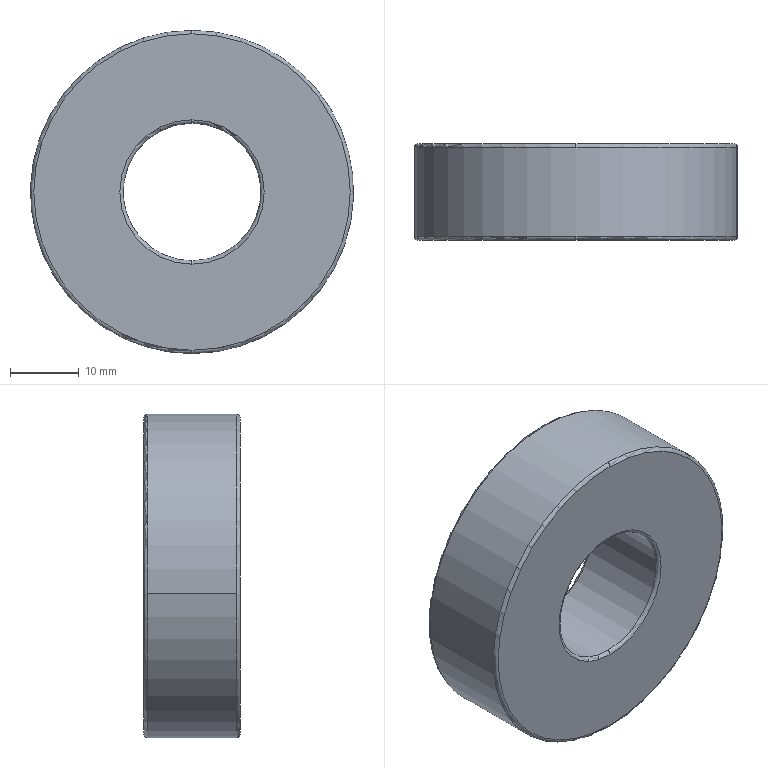Part | SolidWorks | features BaseBody 1 | 1 solid | 14 faces | box 47 x 14 x 47 mm | volume 19868 mm3 | torus 8 | cylinder 4 | plane 2 | commonest cylinder face diameters 20 x2 47 x2
STEP:
#1=CARTESIAN_POINT('',(-530.322,-112.,7.791));
#2=VERTEX_POINT('',#1);
#3=CARTESIAN_POINT('',(-530.322,-112.,28.791));
#4=VERTEX_POINT('',#3);
#5=CARTESIAN_POINT('',(-530.322,-112.,18.291));
#6=DIRECTION('',(0.,1.,0.));
#7=DIRECTION('',(0.,0.,-1.));
#8=AXIS2_PLACEMENT_3D('',#5,#6,#7);
#9=CIRCLE('',#8,10.5);
#10=EDGE_CURVE('',#2,#4,#9,.T.);
#11=ORIENTED_EDGE('',*,*,#10,.F.);
#12=CARTESIAN_POINT('',(-530.322,-111.5,8.291));
#13=VERTEX_POINT('',#12);
#14=CARTESIAN_POINT('',(-530.322,-111.5,7.791));
#15=DIRECTION('',(-1.,0.,0.));
#16=DIRECTION('',(0.,0.,1.));
#17=AXIS2_PLACEMENT_3D('',#14,#15,#16);
#18=CIRCLE('',#17,0.5);
#19=EDGE_CURVE('',#2,#13,#18,.T.);
#20=ORIENTED_EDGE('',*,*,#19,.T.);
#21=CARTESIAN_POINT('',(-540.261,-111.5,17.194));
#22=VERTEX_POINT('',#21);
#23=CARTESIAN_POINT('',(-530.322,-111.5,18.291));
#24=DIRECTION('',(0.,1.,0.));
#25=DIRECTION('',(0.,0.,-1.));
#26=AXIS2_PLACEMENT_3D('',#23,#24,#25);
#27=CIRCLE('',#26,10.);
#28=EDGE_CURVE('',#13,#22,#27,.T.);
#29=ORIENTED_EDGE('',*,*,#28,.T.);
#30=CARTESIAN_POINT('',(-530.322,-111.5,28.291));
#31=VERTEX_POINT('',#30);
#32=CARTESIAN_POINT('',(-530.322,-111.5,18.291));
#33=DIRECTION('',(0.,1.,0.));
#34=DIRECTION('',(0.,0.,-1.));
#35=AXIS2_PLACEMENT_3D('',#32,#33,#34);
#36=CIRCLE('',#35,10.);
#37=EDGE_CURVE('',#22,#31,#36,.T.);
#38=ORIENTED_EDGE('',*,*,#37,.T.);
#39=CARTESIAN_POINT('',(-530.322,-111.5,28.791));
#40=DIRECTION('',(1.,0.,0.));
#41=DIRECTION('',(0.,0.,-1.));
#42=AXIS2_PLACEMENT_3D('',#39,#40,#41);
#43=CIRCLE('',#42,0.5);
#44=EDGE_CURVE('',#4,#31,#43,.T.);
#45=ORIENTED_EDGE('',*,*,#44,.F.);
#46=EDGE_LOOP('',(#11,#20,#29,#38,#45));
#47=FACE_OUTER_BOUND('',#46,.T.);
#48=CARTESIAN_POINT('',(-530.322,-111.5,18.291));
#49=DIRECTION('',(0.,-1.,0.));
#50=DIRECTION('',(0.,0.,1.));
#51=AXIS2_PLACEMENT_3D('',#48,#49,#50);
#52=TOROIDAL_SURFACE('',#51,10.5,0.5);
#53=ADVANCED_FACE('',(#47),#52,.T.);
#54=CARTESIAN_POINT('',(-553.68,-111.5,15.712));
#55=VERTEX_POINT('',#54);
#56=CARTESIAN_POINT('',(-530.322,-111.5,-5.209));
#57=VERTEX_POINT('',#56);
#58=CARTESIAN_POINT('',(-530.322,-111.5,18.291));
#59=DIRECTION('',(0.,-1.,0.));
#60=DIRECTION('',(0.,0.,-1.));
#61=AXIS2_PLACEMENT_3D('',#58,#59,#60);
#62=CIRCLE('',#61,23.5);
#63=EDGE_CURVE('',#55,#57,#62,.T.);
#64=ORIENTED_EDGE('',*,*,#63,.T.);
#65=CARTESIAN_POINT('',(-530.322,-112.,-4.709));
#66=VERTEX_POINT('',#65);
#67=CARTESIAN_POINT('',(-530.322,-111.5,-4.709));
#68=DIRECTION('',(-1.,0.,0.));
#69=DIRECTION('',(0.,0.,1.));
#70=AXIS2_PLACEMENT_3D('',#67,#68,#69);
#71=CIRCLE('',#70,0.5);
#72=EDGE_CURVE('',#57,#66,#71,.T.);
#73=ORIENTED_EDGE('',*,*,#72,.T.);
#74=CARTESIAN_POINT('',(-530.322,-112.,41.291));
#75=VERTEX_POINT('',#74);
#76=CARTESIAN_POINT('',(-530.322,-112.,18.291));
#77=DIRECTION('',(0.,-1.,0.));
#78=DIRECTION('',(0.,0.,-1.));
#79=AXIS2_PLACEMENT_3D('',#76,#77,#78);
#80=CIRCLE('',#79,23.);
#81=EDGE_CURVE('',#75,#66,#80,.T.);
#82=ORIENTED_EDGE('',*,*,#81,.F.);
#83=CARTESIAN_POINT('',(-530.322,-111.5,41.791));
#84=VERTEX_POINT('',#83);
#85=CARTESIAN_POINT('',(-530.322,-111.5,41.291));
#86=DIRECTION('',(1.,0.,0.));
#87=DIRECTION('',(0.,0.,-1.));
#88=AXIS2_PLACEMENT_3D('',#85,#86,#87);
#89=CIRCLE('',#88,0.5);
#90=EDGE_CURVE('',#84,#75,#89,.T.);
#91=ORIENTED_EDGE('',*,*,#90,.F.);
#92=CARTESIAN_POINT('',(-530.322,-111.5,18.291));
#93=DIRECTION('',(0.,-1.,0.));
#94=DIRECTION('',(0.,0.,-1.));
#95=AXIS2_PLACEMENT_3D('',#92,#93,#94);
#96=CIRCLE('',#95,23.5);
#97=EDGE_CURVE('',#84,#55,#96,.T.);
#98=ORIENTED_EDGE('',*,*,#97,.T.);
#99=EDGE_LOOP('',(#64,#73,#82,#91,#98));
#100=FACE_OUTER_BOUND('',#99,.T.);
#101=CARTESIAN_POINT('',(-530.322,-111.5,18.291));
#102=DIRECTION('',(0.,-1.,0.));
#103=DIRECTION('',(0.,0.,1.));
#104=AXIS2_PLACEMENT_3D('',#101,#102,#103);
#105=TOROIDAL_SURFACE('',#104,23.,0.5);
#106=ADVANCED_FACE('',(#100),#105,.T.);
#107=CARTESIAN_POINT('',(-553.68,-98.5,15.712));
#108=VERTEX_POINT('',#107);
#109=CARTESIAN_POINT('',(-530.322,-98.5,41.791));
#110=VERTEX_POINT('',#109);
#111=CARTESIAN_POINT('',(-530.322,-98.5,18.291));
#112=DIRECTION('',(0.,1.,0.));
#113=DIRECTION('',(0.,0.,1.));
#114=AXIS2_PLACEMENT_3D('',#111,#112,#113);
#115=CIRCLE('',#114,23.5);
#116=EDGE_CURVE('',#108,#110,#115,.T.);
#117=ORIENTED_EDGE('',*,*,#116,.T.);
#118=CARTESIAN_POINT('',(-530.322,-98.,41.291));
#119=VERTEX_POINT('',#118);
#120=CARTESIAN_POINT('',(-530.322,-98.5,41.291));
#121=DIRECTION('',(-1.,0.,0.));
#122=DIRECTION('',(0.,0.,1.));
#123=AXIS2_PLACEMENT_3D('',#120,#121,#122);
#124=CIRCLE('',#123,0.5);
#125=EDGE_CURVE('',#110,#119,#124,.T.);
#126=ORIENTED_EDGE('',*,*,#125,.T.);
#127=CARTESIAN_POINT('',(-530.322,-98.,-4.709));
#128=VERTEX_POINT('',#127);
#129=CARTESIAN_POINT('',(-530.322,-98.,18.291));
#130=DIRECTION('',(0.,1.,0.));
#131=DIRECTION('',(0.,0.,1.));
#132=AXIS2_PLACEMENT_3D('',#129,#130,#131);
#133=CIRCLE('',#132,23.);
#134=EDGE_CURVE('',#128,#119,#133,.T.);
#135=ORIENTED_EDGE('',*,*,#134,.F.);
#136=CARTESIAN_POINT('',(-530.322,-98.5,-5.209));
#137=VERTEX_POINT('',#136);
#138=CARTESIAN_POINT('',(-530.322,-98.5,-4.709));
#139=DIRECTION('',(1.,0.,0.));
#140=DIRECTION('',(0.,0.,-1.));
#141=AXIS2_PLACEMENT_3D('',#138,#139,#140);
#142=CIRCLE('',#141,0.5);
#143=EDGE_CURVE('',#137,#128,#142,.T.);
#144=ORIENTED_EDGE('',*,*,#143,.F.);
#145=CARTESIAN_POINT('',(-530.322,-98.5,18.291));
#146=DIRECTION('',(0.,1.,0.));
#147=DIRECTION('',(0.,0.,1.));
#148=AXIS2_PLACEMENT_3D('',#145,#146,#147);
#149=CIRCLE('',#148,23.5);
#150=EDGE_CURVE('',#137,#108,#149,.T.);
#151=ORIENTED_EDGE('',*,*,#150,.T.);
#152=EDGE_LOOP('',(#117,#126,#135,#144,#151));
#153=FACE_OUTER_BOUND('',#152,.T.);
#154=CARTESIAN_POINT('',(-530.322,-98.5,18.291));
#155=DIRECTION('',(0.,1.,0.));
#156=DIRECTION('',(0.,0.,-1.));
#157=AXIS2_PLACEMENT_3D('',#154,#155,#156);
#158=TOROIDAL_SURFACE('',#157,23.,0.5);
#159=ADVANCED_FACE('',(#153),#158,.T.);
#160=CARTESIAN_POINT('',(-530.322,-98.,28.791));
#161=VERTEX_POINT('',#160);
#162=CARTESIAN_POINT('',(-530.322,-98.,7.791));
#163=VERTEX_POINT('',#162);
#164=CARTESIAN_POINT('',(-530.322,-98.,18.291));
#165=DIRECTION('',(0.,-1.,0.));
#166=DIRECTION('',(0.,0.,1.));
#167=AXIS2_PLACEMENT_3D('',#164,#165,#166);
#168=CIRCLE('',#167,10.5);
#169=EDGE_CURVE('',#161,#163,#168,.T.);
#170=ORIENTED_EDGE('',*,*,#169,.F.);
#171=CARTESIAN_POINT('',(-530.322,-98.5,28.291));
#172=VERTEX_POINT('',#171);
#173=CARTESIAN_POINT('',(-530.322,-98.5,28.791));
#174=DIRECTION('',(-1.,0.,0.));
#175=DIRECTION('',(0.,0.,1.));
#176=AXIS2_PLACEMENT_3D('',#173,#174,#175);
#177=CIRCLE('',#176,0.5);
#178=EDGE_CURVE('',#161,#172,#177,.T.);
#179=ORIENTED_EDGE('',*,*,#178,.T.);
#180=CARTESIAN_POINT('',(-540.261,-98.5,17.194));
#181=VERTEX_POINT('',#180);
#182=CARTESIAN_POINT('',(-530.322,-98.5,18.291));
#183=DIRECTION('',(0.,-1.,0.));
#184=DIRECTION('',(0.,0.,1.));
#185=AXIS2_PLACEMENT_3D('',#182,#183,#184);
#186=CIRCLE('',#185,10.);
#187=EDGE_CURVE('',#172,#181,#186,.T.);
#188=ORIENTED_EDGE('',*,*,#187,.T.);
#189=CARTESIAN_POINT('',(-530.322,-98.5,8.291));
#190=VERTEX_POINT('',#189);
#191=CARTESIAN_POINT('',(-530.322,-98.5,18.291));
#192=DIRECTION('',(0.,-1.,0.));
#193=DIRECTION('',(0.,0.,1.));
#194=AXIS2_PLACEMENT_3D('',#191,#192,#193);
#195=CIRCLE('',#194,10.);
#196=EDGE_CURVE('',#181,#190,#195,.T.);
#197=ORIENTED_EDGE('',*,*,#196,.T.);
#198=CARTESIAN_POINT('',(-530.322,-98.5,7.791));
#199=DIRECTION('',(1.,0.,0.));
#200=DIRECTION('',(0.,0.,-1.));
#201=AXIS2_PLACEMENT_3D('',#198,#199,#200);
#202=CIRCLE('',#201,0.5);
#203=EDGE_CURVE('',#163,#190,#202,.T.);
#204=ORIENTED_EDGE('',*,*,#203,.F.);
#205=EDGE_LOOP('',(#170,#179,#188,#197,#204));
#206=FACE_OUTER_BOUND('',#205,.T.);
#207=CARTESIAN_POINT('',(-530.322,-98.5,18.291));
#208=DIRECTION('',(0.,1.,0.));
#209=DIRECTION('',(0.,0.,-1.));
#210=AXIS2_PLACEMENT_3D('',#207,#208,#209);
#211=TOROIDAL_SURFACE('',#210,10.5,0.5);
#212=ADVANCED_FACE('',(#206),#211,.T.);
#213=CARTESIAN_POINT('',(-520.382,-98.5,19.388));
#214=VERTEX_POINT('',#213);
#215=CARTESIAN_POINT('',(-530.322,-98.5,18.291));
#216=DIRECTION('',(0.,-1.,0.));
#217=DIRECTION('',(0.,0.,1.));
#218=AXIS2_PLACEMENT_3D('',#215,#216,#217);
#219=CIRCLE('',#218,10.);
#220=EDGE_CURVE('',#214,#172,#219,.T.);
#221=ORIENTED_EDGE('',*,*,#220,.F.);
#222=CARTESIAN_POINT('',(-520.382,-111.5,19.388));
#223=VERTEX_POINT('',#222);
#224=CARTESIAN_POINT('',(-520.382,-98.,19.388));
#225=DIRECTION('',(0.,-1.,0.));
#226=VECTOR('',#225,1000.);
#227=LINE('',#224,#226);
#228=EDGE_CURVE('',#214,#223,#227,.T.);
#229=ORIENTED_EDGE('',*,*,#228,.T.);
#230=CARTESIAN_POINT('',(-530.322,-111.5,18.291));
#231=DIRECTION('',(0.,1.,0.));
#232=DIRECTION('',(0.,0.,-1.));
#233=AXIS2_PLACEMENT_3D('',#230,#231,#232);
#234=CIRCLE('',#233,10.);
#235=EDGE_CURVE('',#31,#223,#234,.T.);
#236=ORIENTED_EDGE('',*,*,#235,.F.);
#237=ORIENTED_EDGE('',*,*,#37,.F.);
#238=CARTESIAN_POINT('',(-540.261,-98.,17.194));
#239=DIRECTION('',(0.,-1.,0.));
#240=VECTOR('',#239,1000.);
#241=LINE('',#238,#240);
#242=EDGE_CURVE('',#181,#22,#241,.T.);
#243=ORIENTED_EDGE('',*,*,#242,.F.);
#244=ORIENTED_EDGE('',*,*,#187,.F.);
#245=EDGE_LOOP('',(#221,#229,#236,#237,#243,#244));
#246=FACE_OUTER_BOUND('',#245,.T.);
#247=CARTESIAN_POINT('',(-530.322,-98.,18.291));
#248=DIRECTION('',(0.,-1.,0.));
#249=DIRECTION('',(-0.994,0.,-0.1097));
#250=AXIS2_PLACEMENT_3D('',#247,#248,#249);
#251=CYLINDRICAL_SURFACE('',#250,10.);
#252=ADVANCED_FACE('',(#246),#251,.F.);
#253=CARTESIAN_POINT('',(-506.963,-98.5,20.87));
#254=VERTEX_POINT('',#253);
#255=CARTESIAN_POINT('',(-530.322,-98.5,18.291));
#256=DIRECTION('',(0.,1.,0.));
#257=DIRECTION('',(0.,0.,1.));
#258=AXIS2_PLACEMENT_3D('',#255,#256,#257);
#259=CIRCLE('',#258,23.5);
#260=EDGE_CURVE('',#254,#137,#259,.T.);
#261=ORIENTED_EDGE('',*,*,#260,.F.);
#262=CARTESIAN_POINT('',(-506.963,-111.5,20.87));
#263=VERTEX_POINT('',#262);
#264=CARTESIAN_POINT('',(-506.963,-98.,20.87));
#265=DIRECTION('',(0.,-1.,0.));
#266=VECTOR('',#265,1000.);
#267=LINE('',#264,#266);
#268=EDGE_CURVE('',#254,#263,#267,.T.);
#269=ORIENTED_EDGE('',*,*,#268,.T.);
#270=CARTESIAN_POINT('',(-530.322,-111.5,18.291));
#271=DIRECTION('',(0.,-1.,0.));
#272=DIRECTION('',(0.,0.,-1.));
#273=AXIS2_PLACEMENT_3D('',#270,#271,#272);
#274=CIRCLE('',#273,23.5);
#275=EDGE_CURVE('',#57,#263,#274,.T.);
#276=ORIENTED_EDGE('',*,*,#275,.F.);
#277=ORIENTED_EDGE('',*,*,#63,.F.);
#278=CARTESIAN_POINT('',(-553.68,-98.,15.712));
#279=DIRECTION('',(0.,-1.,0.));
#280=VECTOR('',#279,1000.);
#281=LINE('',#278,#280);
#282=EDGE_CURVE('',#108,#55,#281,.T.);
#283=ORIENTED_EDGE('',*,*,#282,.F.);
#284=ORIENTED_EDGE('',*,*,#150,.F.);
#285=EDGE_LOOP('',(#261,#269,#276,#277,#283,#284));
#286=FACE_OUTER_BOUND('',#285,.T.);
#287=CARTESIAN_POINT('',(-530.322,-98.,18.291));
#288=DIRECTION('',(0.,-1.,0.));
#289=DIRECTION('',(-0.994,0.,-0.1097));
#290=AXIS2_PLACEMENT_3D('',#287,#288,#289);
#291=CYLINDRICAL_SURFACE('',#290,23.5);
#292=ADVANCED_FACE('',(#286),#291,.T.);
#293=CARTESIAN_POINT('',(-530.322,-112.,18.291));
#294=DIRECTION('',(0.,1.,0.));
#295=DIRECTION('',(0.,0.,-1.));
#296=AXIS2_PLACEMENT_3D('',#293,#294,#295);
#297=CIRCLE('',#296,10.5);
#298=EDGE_CURVE('',#4,#2,#297,.T.);
#299=ORIENTED_EDGE('',*,*,#298,.T.);
#300=ORIENTED_EDGE('',*,*,#10,.T.);
#301=EDGE_LOOP('',(#299,#300));
#302=FACE_BOUND('',#301,.T.);
#303=ORIENTED_EDGE('',*,*,#81,.T.);
#304=CARTESIAN_POINT('',(-530.322,-112.,18.291));
#305=DIRECTION('',(0.,-1.,0.));
#306=DIRECTION('',(0.,0.,-1.));
#307=AXIS2_PLACEMENT_3D('',#304,#305,#306);
#308=CIRCLE('',#307,23.);
#309=EDGE_CURVE('',#66,#75,#308,.T.);
#310=ORIENTED_EDGE('',*,*,#309,.T.);
#311=EDGE_LOOP('',(#303,#310));
#312=FACE_OUTER_BOUND('',#311,.T.);
#313=CARTESIAN_POINT('',(-530.322,-112.,18.291));
#314=DIRECTION('',(0.,-1.,0.));
#315=DIRECTION('',(0.,0.,-1.));
#316=AXIS2_PLACEMENT_3D('',#313,#314,#315);
#317=PLANE('',#316);
#318=ADVANCED_FACE('',(#302,#312),#317,.T.);
#319=ORIENTED_EDGE('',*,*,#268,.F.);
#320=CARTESIAN_POINT('',(-530.322,-98.5,18.291));
#321=DIRECTION('',(0.,1.,0.));
#322=DIRECTION('',(0.,0.,1.));
#323=AXIS2_PLACEMENT_3D('',#320,#321,#322);
#324=CIRCLE('',#323,23.5);
#325=EDGE_CURVE('',#110,#254,#324,.T.);
#326=ORIENTED_EDGE('',*,*,#325,.F.);
#327=ORIENTED_EDGE('',*,*,#116,.F.);
#328=ORIENTED_EDGE('',*,*,#282,.T.);
#329=ORIENTED_EDGE('',*,*,#97,.F.);
#330=CARTESIAN_POINT('',(-530.322,-111.5,18.291));
#331=DIRECTION('',(0.,-1.,0.));
#332=DIRECTION('',(0.,0.,-1.));
#333=AXIS2_PLACEMENT_3D('',#330,#331,#332);
#334=CIRCLE('',#333,23.5);
#335=EDGE_CURVE('',#263,#84,#334,.T.);
#336=ORIENTED_EDGE('',*,*,#335,.F.);
#337=EDGE_LOOP('',(#319,#326,#327,#328,#329,#336));
#338=FACE_OUTER_BOUND('',#337,.T.);
#339=CARTESIAN_POINT('',(-530.322,-98.,18.291));
#340=DIRECTION('',(0.,-1.,0.));
#341=DIRECTION('',(-0.994,0.,-0.1097));
#342=AXIS2_PLACEMENT_3D('',#339,#340,#341);
#343=CYLINDRICAL_SURFACE('',#342,23.5);
#344=ADVANCED_FACE('',(#338),#343,.T.);
#345=CARTESIAN_POINT('',(-530.322,-98.,18.291));
#346=DIRECTION('',(0.,-1.,0.));
#347=DIRECTION('',(0.,0.,1.));
#348=AXIS2_PLACEMENT_3D('',#345,#346,#347);
#349=CIRCLE('',#348,10.5);
#350=EDGE_CURVE('',#163,#161,#349,.T.);
#351=ORIENTED_EDGE('',*,*,#350,.T.);
#352=ORIENTED_EDGE('',*,*,#169,.T.);
#353=EDGE_LOOP('',(#351,#352));
#354=FACE_BOUND('',#353,.T.);
#355=ORIENTED_EDGE('',*,*,#134,.T.);
#356=CARTESIAN_POINT('',(-530.322,-98.,18.291));
#357=DIRECTION('',(0.,1.,0.));
#358=DIRECTION('',(0.,0.,1.));
#359=AXIS2_PLACEMENT_3D('',#356,#357,#358);
#360=CIRCLE('',#359,23.);
#361=EDGE_CURVE('',#119,#128,#360,.T.);
#362=ORIENTED_EDGE('',*,*,#361,.T.);
#363=EDGE_LOOP('',(#355,#362));
#364=FACE_OUTER_BOUND('',#363,.T.);
#365=CARTESIAN_POINT('',(-530.322,-98.,18.291));
#366=DIRECTION('',(0.,1.,0.));
#367=DIRECTION('',(1.,0.,0.));
#368=AXIS2_PLACEMENT_3D('',#365,#366,#367);
#369=PLANE('',#368);
#370=ADVANCED_FACE('',(#354,#364),#369,.T.);
#371=ORIENTED_EDGE('',*,*,#228,.F.);
#372=CARTESIAN_POINT('',(-530.322,-98.5,18.291));
#373=DIRECTION('',(0.,-1.,0.));
#374=DIRECTION('',(0.,0.,1.));
#375=AXIS2_PLACEMENT_3D('',#372,#373,#374);
#376=CIRCLE('',#375,10.);
#377=EDGE_CURVE('',#190,#214,#376,.T.);
#378=ORIENTED_EDGE('',*,*,#377,.F.);
#379=ORIENTED_EDGE('',*,*,#196,.F.);
#380=ORIENTED_EDGE('',*,*,#242,.T.);
#381=ORIENTED_EDGE('',*,*,#28,.F.);
#382=CARTESIAN_POINT('',(-530.322,-111.5,18.291));
#383=DIRECTION('',(0.,1.,0.));
#384=DIRECTION('',(0.,0.,-1.));
#385=AXIS2_PLACEMENT_3D('',#382,#383,#384);
#386=CIRCLE('',#385,10.);
#387=EDGE_CURVE('',#223,#13,#386,.T.);
#388=ORIENTED_EDGE('',*,*,#387,.F.);
#389=EDGE_LOOP('',(#371,#378,#379,#380,#381,#388));
#390=FACE_OUTER_BOUND('',#389,.T.);
#391=CARTESIAN_POINT('',(-530.322,-98.,18.291));
#392=DIRECTION('',(0.,-1.,0.));
#393=DIRECTION('',(-0.994,0.,-0.1097));
#394=AXIS2_PLACEMENT_3D('',#391,#392,#393);
#395=CYLINDRICAL_SURFACE('',#394,10.);
#396=ADVANCED_FACE('',(#390),#395,.F.);
#397=ORIENTED_EDGE('',*,*,#178,.F.);
#398=ORIENTED_EDGE('',*,*,#350,.F.);
#399=ORIENTED_EDGE('',*,*,#203,.T.);
#400=ORIENTED_EDGE('',*,*,#377,.T.);
#401=ORIENTED_EDGE('',*,*,#220,.T.);
#402=EDGE_LOOP('',(#397,#398,#399,#400,#401));
#403=FACE_OUTER_BOUND('',#402,.T.);
#404=CARTESIAN_POINT('',(-530.322,-98.5,18.291));
#405=DIRECTION('',(0.,1.,0.));
#406=DIRECTION('',(0.,0.,-1.));
#407=AXIS2_PLACEMENT_3D('',#404,#405,#406);
#408=TOROIDAL_SURFACE('',#407,10.5,0.5);
#409=ADVANCED_FACE('',(#403),#408,.T.);
#410=ORIENTED_EDGE('',*,*,#125,.F.);
#411=ORIENTED_EDGE('',*,*,#325,.T.);
#412=ORIENTED_EDGE('',*,*,#260,.T.);
#413=ORIENTED_EDGE('',*,*,#143,.T.);
#414=ORIENTED_EDGE('',*,*,#361,.F.);
#415=EDGE_LOOP('',(#410,#411,#412,#413,#414));
#416=FACE_OUTER_BOUND('',#415,.T.);
#417=CARTESIAN_POINT('',(-530.322,-98.5,18.291));
#418=DIRECTION('',(0.,1.,0.));
#419=DIRECTION('',(0.,0.,-1.));
#420=AXIS2_PLACEMENT_3D('',#417,#418,#419);
#421=TOROIDAL_SURFACE('',#420,23.,0.5);
#422=ADVANCED_FACE('',(#416),#421,.T.);
#423=ORIENTED_EDGE('',*,*,#72,.F.);
#424=ORIENTED_EDGE('',*,*,#275,.T.);
#425=ORIENTED_EDGE('',*,*,#335,.T.);
#426=ORIENTED_EDGE('',*,*,#90,.T.);
#427=ORIENTED_EDGE('',*,*,#309,.F.);
#428=EDGE_LOOP('',(#423,#424,#425,#426,#427));
#429=FACE_OUTER_BOUND('',#428,.T.);
#430=CARTESIAN_POINT('',(-530.322,-111.5,18.291));
#431=DIRECTION('',(0.,-1.,0.));
#432=DIRECTION('',(0.,0.,1.));
#433=AXIS2_PLACEMENT_3D('',#430,#431,#432);
#434=TOROIDAL_SURFACE('',#433,23.,0.5);
#435=ADVANCED_FACE('',(#429),#434,.T.);
#436=ORIENTED_EDGE('',*,*,#19,.F.);
#437=ORIENTED_EDGE('',*,*,#298,.F.);
#438=ORIENTED_EDGE('',*,*,#44,.T.);
#439=ORIENTED_EDGE('',*,*,#235,.T.);
#440=ORIENTED_EDGE('',*,*,#387,.T.);
#441=EDGE_LOOP('',(#436,#437,#438,#439,#440));
#442=FACE_OUTER_BOUND('',#441,.T.);
#443=CARTESIAN_POINT('',(-530.322,-111.5,18.291));
#444=DIRECTION('',(0.,-1.,0.));
#445=DIRECTION('',(0.,0.,1.));
#446=AXIS2_PLACEMENT_3D('',#443,#444,#445);
#447=TOROIDAL_SURFACE('',#446,10.5,0.5);
#448=ADVANCED_FACE('',(#442),#447,.T.);
#449=CLOSED_SHELL('',(#53,#106,#159,#212,#252,#292,#318,#344,#370,#396,#409,#422,#435,#448));
#450=MANIFOLD_SOLID_BREP('',#449);
#451=CARTESIAN_POINT('',(0.,0.,0.));
#452=DIRECTION('',(0.,0.,1.));
#453=DIRECTION('',(1.,0.,0.));
#454=AXIS2_PLACEMENT_3D('',#451,#452,#453);
#455=(LENGTH_UNIT()NAMED_UNIT(*)SI_UNIT(.MILLI.,.METRE.));
#456=UNCERTAINTY_MEASURE_WITH_UNIT(LENGTH_MEASURE(0.00001),#455,'','');
#457=(NAMED_UNIT(*)PLANE_ANGLE_UNIT()SI_UNIT($,.RADIAN.));
#458=(NAMED_UNIT(*)SI_UNIT($,.STERADIAN.)SOLID_ANGLE_UNIT());
#459=(GEOMETRIC_REPRESENTATION_CONTEXT(3)GLOBAL_UNCERTAINTY_ASSIGNED_CONTEXT((#456))GLOBAL_UNIT_ASSIGNED_CONTEXT((#455,#457,#458))REPRESENTATION_CONTEXT('',''));
#460=ADVANCED_BREP_SHAPE_REPRESENTATION('',(#450,#454),#459);